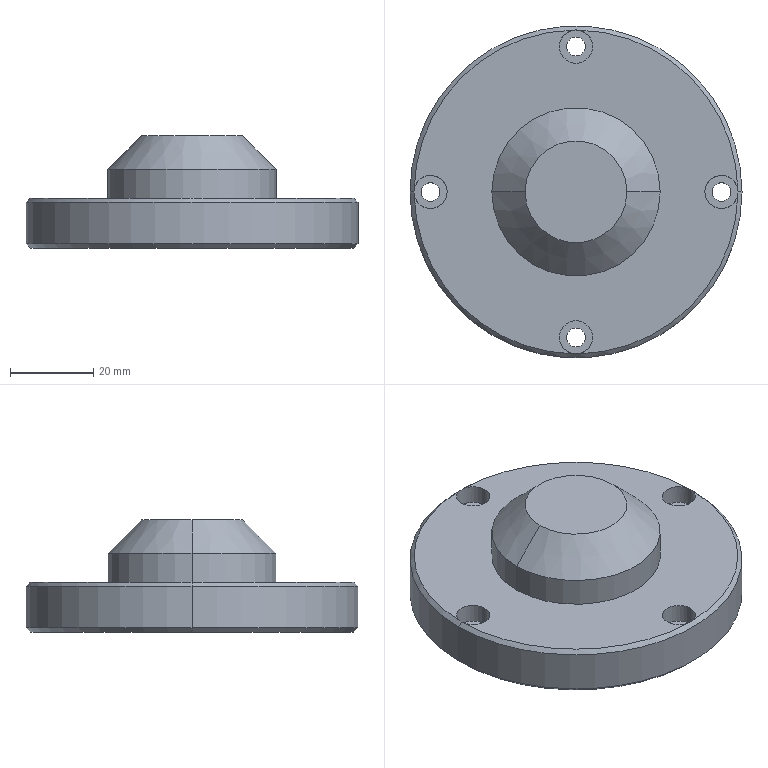Part | STEP file | TJ-DHQM-004-009 | 1 solid | 33 faces | box 79.9 x 79.9 x 27 mm | volume 74312 mm3 | cylinder 20 | plane 7 | cone 6 | commonest cylinder face diameters 4.5 x8 8 x8 40.5 x2 79.9 x2
STEP:
#1=CARTESIAN_POINT('',(12.25,0.,27.));
#2=VERTEX_POINT('',#1);
#3=CARTESIAN_POINT('',(-12.25,0.,27.));
#4=VERTEX_POINT('',#3);
#5=CARTESIAN_POINT('',(0.,0.,27.));
#6=DIRECTION('',(0.,0.,1.));
#7=DIRECTION('',(1.,0.,0.));
#8=AXIS2_PLACEMENT_3D('',#5,#6,#7);
#9=CIRCLE('',#8,12.25);
#10=EDGE_CURVE('',#2,#4,#9,.T.);
#11=ORIENTED_EDGE('',*,*,#10,.F.);
#12=CARTESIAN_POINT('',(20.25,0.,19.));
#13=VERTEX_POINT('',#12);
#14=CARTESIAN_POINT('',(12.25,0.,27.));
#15=DIRECTION('',(0.7071,0.,-0.7071));
#16=VECTOR('',#15,1000.);
#17=LINE('',#14,#16);
#18=EDGE_CURVE('',#2,#13,#17,.T.);
#19=ORIENTED_EDGE('',*,*,#18,.T.);
#20=CARTESIAN_POINT('',(-20.25,0.,19.));
#21=VERTEX_POINT('',#20);
#22=CARTESIAN_POINT('',(0.,0.,19.));
#23=DIRECTION('',(0.,0.,-1.));
#24=DIRECTION('',(1.,0.,0.));
#25=AXIS2_PLACEMENT_3D('',#22,#23,#24);
#26=CIRCLE('',#25,20.25);
#27=EDGE_CURVE('',#21,#13,#26,.T.);
#28=ORIENTED_EDGE('',*,*,#27,.F.);
#29=CARTESIAN_POINT('',(-12.25,0.,27.));
#30=DIRECTION('',(-0.7071,0.,-0.7071));
#31=VECTOR('',#30,1000.);
#32=LINE('',#29,#31);
#33=EDGE_CURVE('',#4,#21,#32,.T.);
#34=ORIENTED_EDGE('',*,*,#33,.F.);
#35=EDGE_LOOP('',(#11,#19,#28,#34));
#36=FACE_OUTER_BOUND('',#35,.T.);
#37=CARTESIAN_POINT('',(0.,0.,27.));
#38=DIRECTION('',(0.,0.,-1.));
#39=DIRECTION('',(-1.,0.,0.));
#40=AXIS2_PLACEMENT_3D('',#37,#38,#39);
#41=CONICAL_SURFACE('',#40,12.25,0.7854);
#42=ADVANCED_FACE('',(#36),#41,.T.);
#43=ORIENTED_EDGE('',*,*,#27,.T.);
#44=CARTESIAN_POINT('',(20.25,0.,12.));
#45=VERTEX_POINT('',#44);
#46=CARTESIAN_POINT('',(20.25,0.,27.));
#47=DIRECTION('',(0.,0.,-1.));
#48=VECTOR('',#47,1000.);
#49=LINE('',#46,#48);
#50=EDGE_CURVE('',#13,#45,#49,.T.);
#51=ORIENTED_EDGE('',*,*,#50,.T.);
#52=CARTESIAN_POINT('',(-20.25,0.,12.));
#53=VERTEX_POINT('',#52);
#54=CARTESIAN_POINT('',(0.,0.,12.));
#55=DIRECTION('',(0.,0.,1.));
#56=DIRECTION('',(1.,0.,0.));
#57=AXIS2_PLACEMENT_3D('',#54,#55,#56);
#58=CIRCLE('',#57,20.25);
#59=EDGE_CURVE('',#45,#53,#58,.T.);
#60=ORIENTED_EDGE('',*,*,#59,.T.);
#61=CARTESIAN_POINT('',(-20.25,0.,27.));
#62=DIRECTION('',(0.,0.,-1.));
#63=VECTOR('',#62,1000.);
#64=LINE('',#61,#63);
#65=EDGE_CURVE('',#21,#53,#64,.T.);
#66=ORIENTED_EDGE('',*,*,#65,.F.);
#67=EDGE_LOOP('',(#43,#51,#60,#66));
#68=FACE_OUTER_BOUND('',#67,.T.);
#69=CARTESIAN_POINT('',(0.,0.,27.));
#70=DIRECTION('',(0.,0.,-1.));
#71=DIRECTION('',(-1.,0.,0.));
#72=AXIS2_PLACEMENT_3D('',#69,#70,#71);
#73=CYLINDRICAL_SURFACE('',#72,20.25);
#74=ADVANCED_FACE('',(#68),#73,.T.);
#75=CARTESIAN_POINT('',(-4.,35.,7.4));
#76=VERTEX_POINT('',#75);
#77=CARTESIAN_POINT('',(4.,35.,7.4));
#78=VERTEX_POINT('',#77);
#79=CARTESIAN_POINT('',(0.,35.,7.4));
#80=DIRECTION('',(0.,0.,1.));
#81=DIRECTION('',(1.,0.,0.));
#82=AXIS2_PLACEMENT_3D('',#79,#80,#81);
#83=CIRCLE('',#82,4.);
#84=EDGE_CURVE('',#76,#78,#83,.T.);
#85=ORIENTED_EDGE('',*,*,#84,.F.);
#86=CARTESIAN_POINT('',(-4.,35.,12.));
#87=VERTEX_POINT('',#86);
#88=CARTESIAN_POINT('',(-4.,35.,12.));
#89=DIRECTION('',(0.,0.,1.));
#90=VECTOR('',#89,1000.);
#91=LINE('',#88,#90);
#92=EDGE_CURVE('',#76,#87,#91,.T.);
#93=ORIENTED_EDGE('',*,*,#92,.T.);
#94=CARTESIAN_POINT('',(4.,35.,12.));
#95=VERTEX_POINT('',#94);
#96=CARTESIAN_POINT('',(0.,35.,12.));
#97=DIRECTION('',(0.,0.,1.));
#98=DIRECTION('',(1.,0.,0.));
#99=AXIS2_PLACEMENT_3D('',#96,#97,#98);
#100=CIRCLE('',#99,4.);
#101=EDGE_CURVE('',#87,#95,#100,.T.);
#102=ORIENTED_EDGE('',*,*,#101,.T.);
#103=CARTESIAN_POINT('',(4.,35.,12.));
#104=DIRECTION('',(0.,0.,1.));
#105=VECTOR('',#104,1000.);
#106=LINE('',#103,#105);
#107=EDGE_CURVE('',#78,#95,#106,.T.);
#108=ORIENTED_EDGE('',*,*,#107,.F.);
#109=EDGE_LOOP('',(#85,#93,#102,#108));
#110=FACE_OUTER_BOUND('',#109,.T.);
#111=CARTESIAN_POINT('',(0.,35.,12.));
#112=DIRECTION('',(0.,0.,1.));
#113=DIRECTION('',(1.,0.,0.));
#114=AXIS2_PLACEMENT_3D('',#111,#112,#113);
#115=CYLINDRICAL_SURFACE('',#114,4.);
#116=ADVANCED_FACE('',(#110),#115,.F.);
#117=CARTESIAN_POINT('',(-2.25,35.,0.));
#118=VERTEX_POINT('',#117);
#119=CARTESIAN_POINT('',(2.25,35.,0.));
#120=VERTEX_POINT('',#119);
#121=CARTESIAN_POINT('',(0.,35.,0.));
#122=DIRECTION('',(0.,0.,1.));
#123=DIRECTION('',(1.,0.,0.));
#124=AXIS2_PLACEMENT_3D('',#121,#122,#123);
#125=CIRCLE('',#124,2.25);
#126=EDGE_CURVE('',#118,#120,#125,.T.);
#127=ORIENTED_EDGE('',*,*,#126,.F.);
#128=CARTESIAN_POINT('',(-2.25,35.,7.4));
#129=VERTEX_POINT('',#128);
#130=CARTESIAN_POINT('',(-2.25,35.,12.));
#131=DIRECTION('',(0.,0.,1.));
#132=VECTOR('',#131,1000.);
#133=LINE('',#130,#132);
#134=EDGE_CURVE('',#118,#129,#133,.T.);
#135=ORIENTED_EDGE('',*,*,#134,.T.);
#136=CARTESIAN_POINT('',(2.25,35.,7.4));
#137=VERTEX_POINT('',#136);
#138=CARTESIAN_POINT('',(0.,35.,7.4));
#139=DIRECTION('',(0.,0.,1.));
#140=DIRECTION('',(1.,0.,0.));
#141=AXIS2_PLACEMENT_3D('',#138,#139,#140);
#142=CIRCLE('',#141,2.25);
#143=EDGE_CURVE('',#129,#137,#142,.T.);
#144=ORIENTED_EDGE('',*,*,#143,.T.);
#145=CARTESIAN_POINT('',(2.25,35.,12.));
#146=DIRECTION('',(0.,0.,1.));
#147=VECTOR('',#146,1000.);
#148=LINE('',#145,#147);
#149=EDGE_CURVE('',#120,#137,#148,.T.);
#150=ORIENTED_EDGE('',*,*,#149,.F.);
#151=EDGE_LOOP('',(#127,#135,#144,#150));
#152=FACE_OUTER_BOUND('',#151,.T.);
#153=CARTESIAN_POINT('',(0.,35.,12.));
#154=DIRECTION('',(0.,0.,1.));
#155=DIRECTION('',(1.,0.,0.));
#156=AXIS2_PLACEMENT_3D('',#153,#154,#155);
#157=CYLINDRICAL_SURFACE('',#156,2.25);
#158=ADVANCED_FACE('',(#152),#157,.F.);
#159=CARTESIAN_POINT('',(-39.,0.,7.4));
#160=VERTEX_POINT('',#159);
#161=CARTESIAN_POINT('',(-31.,0.,7.4));
#162=VERTEX_POINT('',#161);
#163=CARTESIAN_POINT('',(-35.,0.,7.4));
#164=DIRECTION('',(0.,0.,1.));
#165=DIRECTION('',(1.,0.,0.));
#166=AXIS2_PLACEMENT_3D('',#163,#164,#165);
#167=CIRCLE('',#166,4.);
#168=EDGE_CURVE('',#160,#162,#167,.T.);
#169=ORIENTED_EDGE('',*,*,#168,.F.);
#170=CARTESIAN_POINT('',(-39.,0.,11.95));
#171=VERTEX_POINT('',#170);
#172=CARTESIAN_POINT('',(-39.,0.,12.));
#173=DIRECTION('',(0.,0.,1.));
#174=VECTOR('',#173,1000.);
#175=LINE('',#172,#174);
#176=EDGE_CURVE('',#160,#171,#175,.T.);
#177=ORIENTED_EDGE('',*,*,#176,.T.);
#178=CARTESIAN_POINT('',(-38.944,-0.6651,12.));
#179=VERTEX_POINT('',#178);
#180=CARTESIAN_POINT('',(-39.,0.,11.95));
#181=CARTESIAN_POINT('',(-39.,-0.2216,11.95));
#182=CARTESIAN_POINT('',(-38.981,-0.4461,11.967));
#183=CARTESIAN_POINT('',(-38.944,-0.6651,12.));
#184=B_SPLINE_CURVE_WITH_KNOTS('',3,(#180,#181,#182,#183),.UNSPECIFIED.,.F.,.F.,(4,4),(0.0006695,0.001333),.UNSPECIFIED.);
#185=EDGE_CURVE('',#171,#179,#184,.T.);
#186=ORIENTED_EDGE('',*,*,#185,.T.);
#187=CARTESIAN_POINT('',(-31.,0.,12.));
#188=VERTEX_POINT('',#187);
#189=CARTESIAN_POINT('',(-35.,0.,12.));
#190=DIRECTION('',(0.,0.,1.));
#191=DIRECTION('',(1.,0.,0.));
#192=AXIS2_PLACEMENT_3D('',#189,#190,#191);
#193=CIRCLE('',#192,4.);
#194=EDGE_CURVE('',#179,#188,#193,.T.);
#195=ORIENTED_EDGE('',*,*,#194,.T.);
#196=CARTESIAN_POINT('',(-31.,0.,12.));
#197=DIRECTION('',(0.,0.,1.));
#198=VECTOR('',#197,1000.);
#199=LINE('',#196,#198);
#200=EDGE_CURVE('',#162,#188,#199,.T.);
#201=ORIENTED_EDGE('',*,*,#200,.F.);
#202=EDGE_LOOP('',(#169,#177,#186,#195,#201));
#203=FACE_OUTER_BOUND('',#202,.T.);
#204=CARTESIAN_POINT('',(-35.,0.,12.));
#205=DIRECTION('',(0.,0.,1.));
#206=DIRECTION('',(1.,0.,0.));
#207=AXIS2_PLACEMENT_3D('',#204,#205,#206);
#208=CYLINDRICAL_SURFACE('',#207,4.);
#209=ADVANCED_FACE('',(#203),#208,.F.);
#210=CARTESIAN_POINT('',(-37.25,0.,0.));
#211=VERTEX_POINT('',#210);
#212=CARTESIAN_POINT('',(-32.75,0.,0.));
#213=VERTEX_POINT('',#212);
#214=CARTESIAN_POINT('',(-35.,0.,0.));
#215=DIRECTION('',(0.,0.,1.));
#216=DIRECTION('',(1.,0.,0.));
#217=AXIS2_PLACEMENT_3D('',#214,#215,#216);
#218=CIRCLE('',#217,2.25);
#219=EDGE_CURVE('',#211,#213,#218,.T.);
#220=ORIENTED_EDGE('',*,*,#219,.F.);
#221=CARTESIAN_POINT('',(-37.25,0.,7.4));
#222=VERTEX_POINT('',#221);
#223=CARTESIAN_POINT('',(-37.25,0.,12.));
#224=DIRECTION('',(0.,0.,1.));
#225=VECTOR('',#224,1000.);
#226=LINE('',#223,#225);
#227=EDGE_CURVE('',#211,#222,#226,.T.);
#228=ORIENTED_EDGE('',*,*,#227,.T.);
#229=CARTESIAN_POINT('',(-32.75,0.,7.4));
#230=VERTEX_POINT('',#229);
#231=CARTESIAN_POINT('',(-35.,0.,7.4));
#232=DIRECTION('',(0.,0.,1.));
#233=DIRECTION('',(1.,0.,0.));
#234=AXIS2_PLACEMENT_3D('',#231,#232,#233);
#235=CIRCLE('',#234,2.25);
#236=EDGE_CURVE('',#222,#230,#235,.T.);
#237=ORIENTED_EDGE('',*,*,#236,.T.);
#238=CARTESIAN_POINT('',(-32.75,0.,12.));
#239=DIRECTION('',(0.,0.,1.));
#240=VECTOR('',#239,1000.);
#241=LINE('',#238,#240);
#242=EDGE_CURVE('',#213,#230,#241,.T.);
#243=ORIENTED_EDGE('',*,*,#242,.F.);
#244=EDGE_LOOP('',(#220,#228,#237,#243));
#245=FACE_OUTER_BOUND('',#244,.T.);
#246=CARTESIAN_POINT('',(-35.,0.,12.));
#247=DIRECTION('',(0.,0.,1.));
#248=DIRECTION('',(1.,0.,0.));
#249=AXIS2_PLACEMENT_3D('',#246,#247,#248);
#250=CYLINDRICAL_SURFACE('',#249,2.25);
#251=ADVANCED_FACE('',(#245),#250,.F.);
#252=CARTESIAN_POINT('',(-4.,-35.,7.4));
#253=VERTEX_POINT('',#252);
#254=CARTESIAN_POINT('',(4.,-35.,7.4));
#255=VERTEX_POINT('',#254);
#256=CARTESIAN_POINT('',(0.,-35.,7.4));
#257=DIRECTION('',(0.,0.,1.));
#258=DIRECTION('',(1.,0.,0.));
#259=AXIS2_PLACEMENT_3D('',#256,#257,#258);
#260=CIRCLE('',#259,4.);
#261=EDGE_CURVE('',#253,#255,#260,.T.);
#262=ORIENTED_EDGE('',*,*,#261,.F.);
#263=CARTESIAN_POINT('',(-4.,-35.,12.));
#264=VERTEX_POINT('',#263);
#265=CARTESIAN_POINT('',(-4.,-35.,12.));
#266=DIRECTION('',(0.,0.,1.));
#267=VECTOR('',#266,1000.);
#268=LINE('',#265,#267);
#269=EDGE_CURVE('',#253,#264,#268,.T.);
#270=ORIENTED_EDGE('',*,*,#269,.T.);
#271=CARTESIAN_POINT('',(-0.6651,-38.944,12.));
#272=VERTEX_POINT('',#271);
#273=CARTESIAN_POINT('',(0.,-35.,12.));
#274=DIRECTION('',(0.,0.,1.));
#275=DIRECTION('',(1.,0.,0.));
#276=AXIS2_PLACEMENT_3D('',#273,#274,#275);
#277=CIRCLE('',#276,4.);
#278=EDGE_CURVE('',#264,#272,#277,.T.);
#279=ORIENTED_EDGE('',*,*,#278,.T.);
#280=CARTESIAN_POINT('',(0.6651,-38.944,12.));
#281=VERTEX_POINT('',#280);
#282=CARTESIAN_POINT('',(-0.6651,-38.944,12.));
#283=CARTESIAN_POINT('',(-0.4455,-38.981,11.967));
#284=CARTESIAN_POINT('',(-0.2245,-39.,11.95));
#285=CARTESIAN_POINT('',(0.2202,-39.,11.95));
#286=CARTESIAN_POINT('',(0.4454,-38.981,11.967));
#287=CARTESIAN_POINT('',(0.6651,-38.944,12.));
#288=B_SPLINE_CURVE_WITH_KNOTS('',3,(#282,#283,#284,#285,#286,#287),.UNSPECIFIED.,.F.,.F.,(4,2,4),(0.000001333,0.0006674,0.001333),.UNSPECIFIED.);
#289=EDGE_CURVE('',#272,#281,#288,.T.);
#290=ORIENTED_EDGE('',*,*,#289,.T.);
#291=CARTESIAN_POINT('',(4.,-35.,12.));
#292=VERTEX_POINT('',#291);
#293=CARTESIAN_POINT('',(0.,-35.,12.));
#294=DIRECTION('',(0.,0.,1.));
#295=DIRECTION('',(1.,0.,0.));
#296=AXIS2_PLACEMENT_3D('',#293,#294,#295);
#297=CIRCLE('',#296,4.);
#298=EDGE_CURVE('',#281,#292,#297,.T.);
#299=ORIENTED_EDGE('',*,*,#298,.T.);
#300=CARTESIAN_POINT('',(4.,-35.,12.));
#301=DIRECTION('',(0.,0.,1.));
#302=VECTOR('',#301,1000.);
#303=LINE('',#300,#302);
#304=EDGE_CURVE('',#255,#292,#303,.T.);
#305=ORIENTED_EDGE('',*,*,#304,.F.);
#306=EDGE_LOOP('',(#262,#270,#279,#290,#299,#305));
#307=FACE_OUTER_BOUND('',#306,.T.);
#308=CARTESIAN_POINT('',(0.,-35.,12.));
#309=DIRECTION('',(0.,0.,1.));
#310=DIRECTION('',(1.,0.,0.));
#311=AXIS2_PLACEMENT_3D('',#308,#309,#310);
#312=CYLINDRICAL_SURFACE('',#311,4.);
#313=ADVANCED_FACE('',(#307),#312,.F.);
#314=CARTESIAN_POINT('',(-2.25,-35.,0.));
#315=VERTEX_POINT('',#314);
#316=CARTESIAN_POINT('',(2.25,-35.,0.));
#317=VERTEX_POINT('',#316);
#318=CARTESIAN_POINT('',(0.,-35.,0.));
#319=DIRECTION('',(0.,0.,1.));
#320=DIRECTION('',(1.,0.,0.));
#321=AXIS2_PLACEMENT_3D('',#318,#319,#320);
#322=CIRCLE('',#321,2.25);
#323=EDGE_CURVE('',#315,#317,#322,.T.);
#324=ORIENTED_EDGE('',*,*,#323,.F.);
#325=CARTESIAN_POINT('',(-2.25,-35.,7.4));
#326=VERTEX_POINT('',#325);
#327=CARTESIAN_POINT('',(-2.25,-35.,12.));
#328=DIRECTION('',(0.,0.,1.));
#329=VECTOR('',#328,1000.);
#330=LINE('',#327,#329);
#331=EDGE_CURVE('',#315,#326,#330,.T.);
#332=ORIENTED_EDGE('',*,*,#331,.T.);
#333=CARTESIAN_POINT('',(2.25,-35.,7.4));
#334=VERTEX_POINT('',#333);
#335=CARTESIAN_POINT('',(0.,-35.,7.4));
#336=DIRECTION('',(0.,0.,1.));
#337=DIRECTION('',(1.,0.,0.));
#338=AXIS2_PLACEMENT_3D('',#335,#336,#337);
#339=CIRCLE('',#338,2.25);
#340=EDGE_CURVE('',#326,#334,#339,.T.);
#341=ORIENTED_EDGE('',*,*,#340,.T.);
#342=CARTESIAN_POINT('',(2.25,-35.,12.));
#343=DIRECTION('',(0.,0.,1.));
#344=VECTOR('',#343,1000.);
#345=LINE('',#342,#344);
#346=EDGE_CURVE('',#317,#334,#345,.T.);
#347=ORIENTED_EDGE('',*,*,#346,.F.);
#348=EDGE_LOOP('',(#324,#332,#341,#347));
#349=FACE_OUTER_BOUND('',#348,.T.);
#350=CARTESIAN_POINT('',(0.,-35.,12.));
#351=DIRECTION('',(0.,0.,1.));
#352=DIRECTION('',(1.,0.,0.));
#353=AXIS2_PLACEMENT_3D('',#350,#351,#352);
#354=CYLINDRICAL_SURFACE('',#353,2.25);
#355=ADVANCED_FACE('',(#349),#354,.F.);
#356=CARTESIAN_POINT('',(31.,0.,7.4));
#357=VERTEX_POINT('',#356);
#358=CARTESIAN_POINT('',(39.,0.,7.4));
#359=VERTEX_POINT('',#358);
#360=CARTESIAN_POINT('',(35.,0.,7.4));
#361=DIRECTION('',(0.,0.,1.));
#362=DIRECTION('',(1.,0.,0.));
#363=AXIS2_PLACEMENT_3D('',#360,#361,#362);
#364=CIRCLE('',#363,4.);
#365=EDGE_CURVE('',#357,#359,#364,.T.);
#366=ORIENTED_EDGE('',*,*,#365,.F.);
#367=CARTESIAN_POINT('',(31.,0.,12.));
#368=VERTEX_POINT('',#367);
#369=CARTESIAN_POINT('',(31.,0.,12.));
#370=DIRECTION('',(0.,0.,1.));
#371=VECTOR('',#370,1000.);
#372=LINE('',#369,#371);
#373=EDGE_CURVE('',#357,#368,#372,.T.);
#374=ORIENTED_EDGE('',*,*,#373,.T.);
#375=CARTESIAN_POINT('',(38.944,-0.6651,12.));
#376=VERTEX_POINT('',#375);
#377=CARTESIAN_POINT('',(35.,0.,12.));
#378=DIRECTION('',(0.,0.,1.));
#379=DIRECTION('',(1.,0.,0.));
#380=AXIS2_PLACEMENT_3D('',#377,#378,#379);
#381=CIRCLE('',#380,4.);
#382=EDGE_CURVE('',#368,#376,#381,.T.);
#383=ORIENTED_EDGE('',*,*,#382,.T.);
#384=CARTESIAN_POINT('',(39.,0.,11.95));
#385=VERTEX_POINT('',#384);
#386=CARTESIAN_POINT('',(38.944,-0.6651,12.));
#387=CARTESIAN_POINT('',(38.981,-0.4448,11.967));
#388=CARTESIAN_POINT('',(39.,-0.2231,11.95));
#389=CARTESIAN_POINT('',(39.,0.,11.95));
#390=B_SPLINE_CURVE_WITH_KNOTS('',3,(#386,#387,#388,#389),.UNSPECIFIED.,.F.,.F.,(4,4),(0.000001333,0.0006695),.UNSPECIFIED.);
#391=EDGE_CURVE('',#376,#385,#390,.T.);
#392=ORIENTED_EDGE('',*,*,#391,.T.);
#393=CARTESIAN_POINT('',(39.,0.,12.));
#394=DIRECTION('',(0.,0.,1.));
#395=VECTOR('',#394,1000.);
#396=LINE('',#393,#395);
#397=EDGE_CURVE('',#359,#385,#396,.T.);
#398=ORIENTED_EDGE('',*,*,#397,.F.);
#399=EDGE_LOOP('',(#366,#374,#383,#392,#398));
#400=FACE_OUTER_BOUND('',#399,.T.);
#401=CARTESIAN_POINT('',(35.,0.,12.));
#402=DIRECTION('',(0.,0.,1.));
#403=DIRECTION('',(1.,0.,0.));
#404=AXIS2_PLACEMENT_3D('',#401,#402,#403);
#405=CYLINDRICAL_SURFACE('',#404,4.);
#406=ADVANCED_FACE('',(#400),#405,.F.);
#407=CARTESIAN_POINT('',(32.75,0.,0.));
#408=VERTEX_POINT('',#407);
#409=CARTESIAN_POINT('',(37.25,0.,0.));
#410=VERTEX_POINT('',#409);
#411=CARTESIAN_POINT('',(35.,0.,0.));
#412=DIRECTION('',(0.,0.,1.));
#413=DIRECTION('',(1.,0.,0.));
#414=AXIS2_PLACEMENT_3D('',#411,#412,#413);
#415=CIRCLE('',#414,2.25);
#416=EDGE_CURVE('',#408,#410,#415,.T.);
#417=ORIENTED_EDGE('',*,*,#416,.F.);
#418=CARTESIAN_POINT('',(32.75,0.,7.4));
#419=VERTEX_POINT('',#418);
#420=CARTESIAN_POINT('',(32.75,0.,12.));
#421=DIRECTION('',(0.,0.,1.));
#422=VECTOR('',#421,1000.);
#423=LINE('',#420,#422);
#424=EDGE_CURVE('',#408,#419,#423,.T.);
#425=ORIENTED_EDGE('',*,*,#424,.T.);
#426=CARTESIAN_POINT('',(37.25,0.,7.4));
#427=VERTEX_POINT('',#426);
#428=CARTESIAN_POINT('',(35.,0.,7.4));
#429=DIRECTION('',(0.,0.,1.));
#430=DIRECTION('',(1.,0.,0.));
#431=AXIS2_PLACEMENT_3D('',#428,#429,#430);
#432=CIRCLE('',#431,2.25);
#433=EDGE_CURVE('',#419,#427,#432,.T.);
#434=ORIENTED_EDGE('',*,*,#433,.T.);
#435=CARTESIAN_POINT('',(37.25,0.,12.));
#436=DIRECTION('',(0.,0.,1.));
#437=VECTOR('',#436,1000.);
#438=LINE('',#435,#437);
#439=EDGE_CURVE('',#410,#427,#438,.T.);
#440=ORIENTED_EDGE('',*,*,#439,.F.);
#441=EDGE_LOOP('',(#417,#425,#434,#440));
#442=FACE_OUTER_BOUND('',#441,.T.);
#443=CARTESIAN_POINT('',(35.,0.,12.));
#444=DIRECTION('',(0.,0.,1.));
#445=DIRECTION('',(1.,0.,0.));
#446=AXIS2_PLACEMENT_3D('',#443,#444,#445);
#447=CYLINDRICAL_SURFACE('',#446,2.25);
#448=ADVANCED_FACE('',(#442),#447,.F.);
#449=CARTESIAN_POINT('',(38.944,0.6651,12.));
#450=VERTEX_POINT('',#449);
#451=CARTESIAN_POINT('',(39.,0.,11.95));
#452=CARTESIAN_POINT('',(39.,0.2216,11.95));
#453=CARTESIAN_POINT('',(38.981,0.4461,11.967));
#454=CARTESIAN_POINT('',(38.944,0.6651,12.));
#455=B_SPLINE_CURVE_WITH_KNOTS('',3,(#451,#452,#453,#454),.UNSPECIFIED.,.F.,.F.,(4,4),(0.0006695,0.001333),.UNSPECIFIED.);
#456=EDGE_CURVE('',#385,#450,#455,.T.);
#457=ORIENTED_EDGE('',*,*,#456,.F.);
#458=CARTESIAN_POINT('',(39.95,0.,11.));
#459=VERTEX_POINT('',#458);
#460=CARTESIAN_POINT('',(38.95,0.,12.));
#461=DIRECTION('',(0.7071,0.,-0.7071));
#462=VECTOR('',#461,1000.);
#463=LINE('',#460,#462);
#464=EDGE_CURVE('',#385,#459,#463,.T.);
#465=ORIENTED_EDGE('',*,*,#464,.T.);
#466=CARTESIAN_POINT('',(-39.95,0.,11.));
#467=VERTEX_POINT('',#466);
#468=CARTESIAN_POINT('',(0.,0.,11.));
#469=DIRECTION('',(0.,0.,-1.));
#470=DIRECTION('',(1.,0.,0.));
#471=AXIS2_PLACEMENT_3D('',#468,#469,#470);
#472=CIRCLE('',#471,39.95);
#473=EDGE_CURVE('',#467,#459,#472,.T.);
#474=ORIENTED_EDGE('',*,*,#473,.F.);
#475=CARTESIAN_POINT('',(-38.95,0.,12.));
#476=DIRECTION('',(-0.7071,0.,-0.7071));
#477=VECTOR('',#476,1000.);
#478=LINE('',#475,#477);
#479=EDGE_CURVE('',#171,#467,#478,.T.);
#480=ORIENTED_EDGE('',*,*,#479,.F.);
#481=CARTESIAN_POINT('',(-38.944,0.6651,12.));
#482=VERTEX_POINT('',#481);
#483=CARTESIAN_POINT('',(-38.944,0.6651,12.));
#484=CARTESIAN_POINT('',(-38.981,0.4448,11.967));
#485=CARTESIAN_POINT('',(-39.,0.2231,11.95));
#486=CARTESIAN_POINT('',(-39.,0.,11.95));
#487=B_SPLINE_CURVE_WITH_KNOTS('',3,(#483,#484,#485,#486),.UNSPECIFIED.,.F.,.F.,(4,4),(0.000001333,0.0006695),.UNSPECIFIED.);
#488=EDGE_CURVE('',#482,#171,#487,.T.);
#489=ORIENTED_EDGE('',*,*,#488,.F.);
#490=CARTESIAN_POINT('',(-0.6651,38.944,12.));
#491=VERTEX_POINT('',#490);
#492=CARTESIAN_POINT('',(0.,0.,12.));
#493=DIRECTION('',(0.,0.,1.));
#494=DIRECTION('',(1.,0.,0.));
#495=AXIS2_PLACEMENT_3D('',#492,#493,#494);
#496=CIRCLE('',#495,38.95);
#497=EDGE_CURVE('',#491,#482,#496,.T.);
#498=ORIENTED_EDGE('',*,*,#497,.F.);
#499=CARTESIAN_POINT('',(0.6651,38.944,12.));
#500=VERTEX_POINT('',#499);
#501=CARTESIAN_POINT('',(0.6651,38.944,12.));
#502=CARTESIAN_POINT('',(0.4455,38.981,11.967));
#503=CARTESIAN_POINT('',(0.2245,39.,11.95));
#504=CARTESIAN_POINT('',(-0.2202,39.,11.95));
#505=CARTESIAN_POINT('',(-0.4454,38.981,11.967));
#506=CARTESIAN_POINT('',(-0.6651,38.944,12.));
#507=B_SPLINE_CURVE_WITH_KNOTS('',3,(#501,#502,#503,#504,#505,#506),.UNSPECIFIED.,.F.,.F.,(4,2,4),(0.000001333,0.0006674,0.001333),.UNSPECIFIED.);
#508=EDGE_CURVE('',#500,#491,#507,.T.);
#509=ORIENTED_EDGE('',*,*,#508,.F.);
#510=CARTESIAN_POINT('',(0.,0.,12.));
#511=DIRECTION('',(0.,0.,1.));
#512=DIRECTION('',(1.,0.,0.));
#513=AXIS2_PLACEMENT_3D('',#510,#511,#512);
#514=CIRCLE('',#513,38.95);
#515=EDGE_CURVE('',#450,#500,#514,.T.);
#516=ORIENTED_EDGE('',*,*,#515,.F.);
#517=EDGE_LOOP('',(#457,#465,#474,#480,#489,#498,#509,#516));
#518=FACE_OUTER_BOUND('',#517,.T.);
#519=CARTESIAN_POINT('',(0.,0.,12.));
#520=DIRECTION('',(0.,0.,-1.));
#521=DIRECTION('',(-1.,0.,0.));
#522=AXIS2_PLACEMENT_3D('',#519,#520,#521);
#523=CONICAL_SURFACE('',#522,38.95,0.7854);
#524=ADVANCED_FACE('',(#518),#523,.T.);
#525=CARTESIAN_POINT('',(-38.95,0.,0.));
#526=VERTEX_POINT('',#525);
#527=CARTESIAN_POINT('',(38.95,0.,0.));
#528=VERTEX_POINT('',#527);
#529=CARTESIAN_POINT('',(0.,0.,0.));
#530=DIRECTION('',(0.,0.,-1.));
#531=DIRECTION('',(1.,0.,0.));
#532=AXIS2_PLACEMENT_3D('',#529,#530,#531);
#533=CIRCLE('',#532,38.95);
#534=EDGE_CURVE('',#526,#528,#533,.T.);
#535=ORIENTED_EDGE('',*,*,#534,.F.);
#536=CARTESIAN_POINT('',(-39.95,0.,1.));
#537=VERTEX_POINT('',#536);
#538=CARTESIAN_POINT('',(-39.95,0.,1.));
#539=DIRECTION('',(-0.7071,0.,0.7071));
#540=VECTOR('',#539,1000.);
#541=LINE('',#538,#540);
#542=EDGE_CURVE('',#526,#537,#541,.T.);
#543=ORIENTED_EDGE('',*,*,#542,.T.);
#544=CARTESIAN_POINT('',(39.95,0.,1.));
#545=VERTEX_POINT('',#544);
#546=CARTESIAN_POINT('',(0.,0.,1.));
#547=DIRECTION('',(0.,0.,1.));
#548=DIRECTION('',(1.,0.,0.));
#549=AXIS2_PLACEMENT_3D('',#546,#547,#548);
#550=CIRCLE('',#549,39.95);
#551=EDGE_CURVE('',#545,#537,#550,.T.);
#552=ORIENTED_EDGE('',*,*,#551,.F.);
#553=CARTESIAN_POINT('',(39.95,0.,1.));
#554=DIRECTION('',(0.7071,0.,0.7071));
#555=VECTOR('',#554,1000.);
#556=LINE('',#553,#555);
#557=EDGE_CURVE('',#528,#545,#556,.T.);
#558=ORIENTED_EDGE('',*,*,#557,.F.);
#559=EDGE_LOOP('',(#535,#543,#552,#558));
#560=FACE_OUTER_BOUND('',#559,.T.);
#561=CARTESIAN_POINT('',(0.,0.,1.));
#562=DIRECTION('',(0.,0.,1.));
#563=DIRECTION('',(1.,0.,0.));
#564=AXIS2_PLACEMENT_3D('',#561,#562,#563);
#565=CONICAL_SURFACE('',#564,39.95,0.7854);
#566=ADVANCED_FACE('',(#560),#565,.T.);
#567=ORIENTED_EDGE('',*,*,#473,.T.);
#568=CARTESIAN_POINT('',(39.95,0.,12.));
#569=DIRECTION('',(0.,0.,-1.));
#570=VECTOR('',#569,1000.);
#571=LINE('',#568,#570);
#572=EDGE_CURVE('',#459,#545,#571,.T.);
#573=ORIENTED_EDGE('',*,*,#572,.T.);
#574=ORIENTED_EDGE('',*,*,#551,.T.);
#575=CARTESIAN_POINT('',(-39.95,0.,12.));
#576=DIRECTION('',(0.,0.,-1.));
#577=VECTOR('',#576,1000.);
#578=LINE('',#575,#577);
#579=EDGE_CURVE('',#467,#537,#578,.T.);
#580=ORIENTED_EDGE('',*,*,#579,.F.);
#581=EDGE_LOOP('',(#567,#573,#574,#580));
#582=FACE_OUTER_BOUND('',#581,.T.);
#583=CARTESIAN_POINT('',(0.,0.,12.));
#584=DIRECTION('',(0.,0.,-1.));
#585=DIRECTION('',(-1.,0.,0.));
#586=AXIS2_PLACEMENT_3D('',#583,#584,#585);
#587=CYLINDRICAL_SURFACE('',#586,39.95);
#588=ADVANCED_FACE('',(#582),#587,.T.);
#589=ORIENTED_EDGE('',*,*,#572,.F.);
#590=CARTESIAN_POINT('',(0.,0.,11.));
#591=DIRECTION('',(0.,0.,-1.));
#592=DIRECTION('',(1.,0.,0.));
#593=AXIS2_PLACEMENT_3D('',#590,#591,#592);
#594=CIRCLE('',#593,39.95);
#595=EDGE_CURVE('',#459,#467,#594,.T.);
#596=ORIENTED_EDGE('',*,*,#595,.T.);
#597=ORIENTED_EDGE('',*,*,#579,.T.);
#598=CARTESIAN_POINT('',(0.,0.,1.));
#599=DIRECTION('',(0.,0.,1.));
#600=DIRECTION('',(1.,0.,0.));
#601=AXIS2_PLACEMENT_3D('',#598,#599,#600);
#602=CIRCLE('',#601,39.95);
#603=EDGE_CURVE('',#537,#545,#602,.T.);
#604=ORIENTED_EDGE('',*,*,#603,.T.);
#605=EDGE_LOOP('',(#589,#596,#597,#604));
#606=FACE_OUTER_BOUND('',#605,.T.);
#607=CARTESIAN_POINT('',(0.,0.,12.));
#608=DIRECTION('',(0.,0.,-1.));
#609=DIRECTION('',(-1.,0.,0.));
#610=AXIS2_PLACEMENT_3D('',#607,#608,#609);
#611=CYLINDRICAL_SURFACE('',#610,39.95);
#612=ADVANCED_FACE('',(#606),#611,.T.);
#613=CARTESIAN_POINT('',(0.,0.,12.));
#614=DIRECTION('',(0.,0.,1.));
#615=DIRECTION('',(1.,0.,0.));
#616=AXIS2_PLACEMENT_3D('',#613,#614,#615);
#617=CIRCLE('',#616,20.25);
#618=EDGE_CURVE('',#53,#45,#617,.T.);
#619=ORIENTED_EDGE('',*,*,#618,.F.);
#620=ORIENTED_EDGE('',*,*,#59,.F.);
#621=EDGE_LOOP('',(#619,#620));
#622=FACE_BOUND('',#621,.T.);
#623=CARTESIAN_POINT('',(0.,35.,12.));
#624=DIRECTION('',(0.,0.,1.));
#625=DIRECTION('',(1.,0.,0.));
#626=AXIS2_PLACEMENT_3D('',#623,#624,#625);
#627=CIRCLE('',#626,4.);
#628=EDGE_CURVE('',#491,#87,#627,.T.);
#629=ORIENTED_EDGE('',*,*,#628,.F.);
#630=ORIENTED_EDGE('',*,*,#497,.T.);
#631=CARTESIAN_POINT('',(-35.,0.,12.));
#632=DIRECTION('',(0.,0.,1.));
#633=DIRECTION('',(1.,0.,0.));
#634=AXIS2_PLACEMENT_3D('',#631,#632,#633);
#635=CIRCLE('',#634,4.);
#636=EDGE_CURVE('',#188,#482,#635,.T.);
#637=ORIENTED_EDGE('',*,*,#636,.F.);
#638=ORIENTED_EDGE('',*,*,#194,.F.);
#639=CARTESIAN_POINT('',(0.,0.,12.));
#640=DIRECTION('',(0.,0.,1.));
#641=DIRECTION('',(1.,0.,0.));
#642=AXIS2_PLACEMENT_3D('',#639,#640,#641);
#643=CIRCLE('',#642,38.95);
#644=EDGE_CURVE('',#179,#272,#643,.T.);
#645=ORIENTED_EDGE('',*,*,#644,.T.);
#646=ORIENTED_EDGE('',*,*,#278,.F.);
#647=CARTESIAN_POINT('',(0.,-35.,12.));
#648=DIRECTION('',(0.,0.,1.));
#649=DIRECTION('',(1.,0.,0.));
#650=AXIS2_PLACEMENT_3D('',#647,#648,#649);
#651=CIRCLE('',#650,4.);
#652=EDGE_CURVE('',#292,#264,#651,.T.);
#653=ORIENTED_EDGE('',*,*,#652,.F.);
#654=ORIENTED_EDGE('',*,*,#298,.F.);
#655=CARTESIAN_POINT('',(0.,0.,12.));
#656=DIRECTION('',(0.,0.,1.));
#657=DIRECTION('',(1.,0.,0.));
#658=AXIS2_PLACEMENT_3D('',#655,#656,#657);
#659=CIRCLE('',#658,38.95);
#660=EDGE_CURVE('',#281,#376,#659,.T.);
#661=ORIENTED_EDGE('',*,*,#660,.T.);
#662=ORIENTED_EDGE('',*,*,#382,.F.);
#663=CARTESIAN_POINT('',(35.,0.,12.));
#664=DIRECTION('',(0.,0.,1.));
#665=DIRECTION('',(1.,0.,0.));
#666=AXIS2_PLACEMENT_3D('',#663,#664,#665);
#667=CIRCLE('',#666,4.);
#668=EDGE_CURVE('',#450,#368,#667,.T.);
#669=ORIENTED_EDGE('',*,*,#668,.F.);
#670=ORIENTED_EDGE('',*,*,#515,.T.);
#671=CARTESIAN_POINT('',(0.,35.,12.));
#672=DIRECTION('',(0.,0.,1.));
#673=DIRECTION('',(1.,0.,0.));
#674=AXIS2_PLACEMENT_3D('',#671,#672,#673);
#675=CIRCLE('',#674,4.);
#676=EDGE_CURVE('',#95,#500,#675,.T.);
#677=ORIENTED_EDGE('',*,*,#676,.F.);
#678=ORIENTED_EDGE('',*,*,#101,.F.);
#679=EDGE_LOOP('',(#629,#630,#637,#638,#645,#646,#653,#654,#661,#662,#669,#670,#677,#678));
#680=FACE_OUTER_BOUND('',#679,.T.);
#681=CARTESIAN_POINT('',(0.,0.,12.));
#682=DIRECTION('',(0.,0.,1.));
#683=DIRECTION('',(1.,0.,0.));
#684=AXIS2_PLACEMENT_3D('',#681,#682,#683);
#685=PLANE('',#684);
#686=ADVANCED_FACE('',(#622,#680),#685,.T.);
#687=CARTESIAN_POINT('',(0.,35.,0.));
#688=DIRECTION('',(0.,0.,1.));
#689=DIRECTION('',(1.,0.,0.));
#690=AXIS2_PLACEMENT_3D('',#687,#688,#689);
#691=CIRCLE('',#690,2.25);
#692=EDGE_CURVE('',#120,#118,#691,.T.);
#693=ORIENTED_EDGE('',*,*,#692,.T.);
#694=ORIENTED_EDGE('',*,*,#126,.T.);
#695=EDGE_LOOP('',(#693,#694));
#696=FACE_BOUND('',#695,.T.);
#697=CARTESIAN_POINT('',(-35.,0.,0.));
#698=DIRECTION('',(0.,0.,1.));
#699=DIRECTION('',(1.,0.,0.));
#700=AXIS2_PLACEMENT_3D('',#697,#698,#699);
#701=CIRCLE('',#700,2.25);
#702=EDGE_CURVE('',#213,#211,#701,.T.);
#703=ORIENTED_EDGE('',*,*,#702,.T.);
#704=ORIENTED_EDGE('',*,*,#219,.T.);
#705=EDGE_LOOP('',(#703,#704));
#706=FACE_BOUND('',#705,.T.);
#707=CARTESIAN_POINT('',(0.,-35.,0.));
#708=DIRECTION('',(0.,0.,1.));
#709=DIRECTION('',(1.,0.,0.));
#710=AXIS2_PLACEMENT_3D('',#707,#708,#709);
#711=CIRCLE('',#710,2.25);
#712=EDGE_CURVE('',#317,#315,#711,.T.);
#713=ORIENTED_EDGE('',*,*,#712,.T.);
#714=ORIENTED_EDGE('',*,*,#323,.T.);
#715=EDGE_LOOP('',(#713,#714));
#716=FACE_BOUND('',#715,.T.);
#717=CARTESIAN_POINT('',(35.,0.,0.));
#718=DIRECTION('',(0.,0.,1.));
#719=DIRECTION('',(1.,0.,0.));
#720=AXIS2_PLACEMENT_3D('',#717,#718,#719);
#721=CIRCLE('',#720,2.25);
#722=EDGE_CURVE('',#410,#408,#721,.T.);
#723=ORIENTED_EDGE('',*,*,#722,.T.);
#724=ORIENTED_EDGE('',*,*,#416,.T.);
#725=EDGE_LOOP('',(#723,#724));
#726=FACE_BOUND('',#725,.T.);
#727=CARTESIAN_POINT('',(0.,0.,0.));
#728=DIRECTION('',(0.,0.,-1.));
#729=DIRECTION('',(1.,0.,0.));
#730=AXIS2_PLACEMENT_3D('',#727,#728,#729);
#731=CIRCLE('',#730,38.95);
#732=EDGE_CURVE('',#528,#526,#731,.T.);
#733=ORIENTED_EDGE('',*,*,#732,.T.);
#734=ORIENTED_EDGE('',*,*,#534,.T.);
#735=EDGE_LOOP('',(#733,#734));
#736=FACE_OUTER_BOUND('',#735,.T.);
#737=CARTESIAN_POINT('',(0.,0.,0.));
#738=DIRECTION('',(0.,0.,1.));
#739=DIRECTION('',(1.,0.,0.));
#740=AXIS2_PLACEMENT_3D('',#737,#738,#739);
#741=PLANE('',#740);
#742=ADVANCED_FACE('',(#696,#706,#716,#726,#736),#741,.F.);
#743=ORIENTED_EDGE('',*,*,#542,.F.);
#744=ORIENTED_EDGE('',*,*,#732,.F.);
#745=ORIENTED_EDGE('',*,*,#557,.T.);
#746=ORIENTED_EDGE('',*,*,#603,.F.);
#747=EDGE_LOOP('',(#743,#744,#745,#746));
#748=FACE_OUTER_BOUND('',#747,.T.);
#749=CARTESIAN_POINT('',(0.,0.,1.));
#750=DIRECTION('',(0.,0.,1.));
#751=DIRECTION('',(1.,0.,0.));
#752=AXIS2_PLACEMENT_3D('',#749,#750,#751);
#753=CONICAL_SURFACE('',#752,39.95,0.7854);
#754=ADVANCED_FACE('',(#748),#753,.T.);
#755=ORIENTED_EDGE('',*,*,#464,.F.);
#756=ORIENTED_EDGE('',*,*,#391,.F.);
#757=ORIENTED_EDGE('',*,*,#660,.F.);
#758=ORIENTED_EDGE('',*,*,#289,.F.);
#759=ORIENTED_EDGE('',*,*,#644,.F.);
#760=ORIENTED_EDGE('',*,*,#185,.F.);
#761=ORIENTED_EDGE('',*,*,#479,.T.);
#762=ORIENTED_EDGE('',*,*,#595,.F.);
#763=EDGE_LOOP('',(#755,#756,#757,#758,#759,#760,#761,#762));
#764=FACE_OUTER_BOUND('',#763,.T.);
#765=CARTESIAN_POINT('',(0.,0.,12.));
#766=DIRECTION('',(0.,0.,-1.));
#767=DIRECTION('',(-1.,0.,0.));
#768=AXIS2_PLACEMENT_3D('',#765,#766,#767);
#769=CONICAL_SURFACE('',#768,38.95,0.7854);
#770=ADVANCED_FACE('',(#764),#769,.T.);
#771=ORIENTED_EDGE('',*,*,#424,.F.);
#772=ORIENTED_EDGE('',*,*,#722,.F.);
#773=ORIENTED_EDGE('',*,*,#439,.T.);
#774=CARTESIAN_POINT('',(35.,0.,7.4));
#775=DIRECTION('',(0.,0.,1.));
#776=DIRECTION('',(1.,0.,0.));
#777=AXIS2_PLACEMENT_3D('',#774,#775,#776);
#778=CIRCLE('',#777,2.25);
#779=EDGE_CURVE('',#427,#419,#778,.T.);
#780=ORIENTED_EDGE('',*,*,#779,.T.);
#781=EDGE_LOOP('',(#771,#772,#773,#780));
#782=FACE_OUTER_BOUND('',#781,.T.);
#783=CARTESIAN_POINT('',(35.,0.,12.));
#784=DIRECTION('',(0.,0.,1.));
#785=DIRECTION('',(1.,0.,0.));
#786=AXIS2_PLACEMENT_3D('',#783,#784,#785);
#787=CYLINDRICAL_SURFACE('',#786,2.25);
#788=ADVANCED_FACE('',(#782),#787,.F.);
#789=ORIENTED_EDGE('',*,*,#779,.F.);
#790=ORIENTED_EDGE('',*,*,#433,.F.);
#791=EDGE_LOOP('',(#789,#790));
#792=FACE_BOUND('',#791,.T.);
#793=CARTESIAN_POINT('',(35.,0.,7.4));
#794=DIRECTION('',(0.,0.,1.));
#795=DIRECTION('',(1.,0.,0.));
#796=AXIS2_PLACEMENT_3D('',#793,#794,#795);
#797=CIRCLE('',#796,4.);
#798=EDGE_CURVE('',#359,#357,#797,.T.);
#799=ORIENTED_EDGE('',*,*,#798,.T.);
#800=ORIENTED_EDGE('',*,*,#365,.T.);
#801=EDGE_LOOP('',(#799,#800));
#802=FACE_OUTER_BOUND('',#801,.T.);
#803=CARTESIAN_POINT('',(37.25,0.,7.4));
#804=DIRECTION('',(0.,0.,-1.));
#805=DIRECTION('',(-1.,0.,0.));
#806=AXIS2_PLACEMENT_3D('',#803,#804,#805);
#807=PLANE('',#806);
#808=ADVANCED_FACE('',(#792,#802),#807,.F.);
#809=ORIENTED_EDGE('',*,*,#373,.F.);
#810=ORIENTED_EDGE('',*,*,#798,.F.);
#811=ORIENTED_EDGE('',*,*,#397,.T.);
#812=ORIENTED_EDGE('',*,*,#456,.T.);
#813=ORIENTED_EDGE('',*,*,#668,.T.);
#814=EDGE_LOOP('',(#809,#810,#811,#812,#813));
#815=FACE_OUTER_BOUND('',#814,.T.);
#816=CARTESIAN_POINT('',(35.,0.,12.));
#817=DIRECTION('',(0.,0.,1.));
#818=DIRECTION('',(1.,0.,0.));
#819=AXIS2_PLACEMENT_3D('',#816,#817,#818);
#820=CYLINDRICAL_SURFACE('',#819,4.);
#821=ADVANCED_FACE('',(#815),#820,.F.);
#822=ORIENTED_EDGE('',*,*,#331,.F.);
#823=ORIENTED_EDGE('',*,*,#712,.F.);
#824=ORIENTED_EDGE('',*,*,#346,.T.);
#825=CARTESIAN_POINT('',(0.,-35.,7.4));
#826=DIRECTION('',(0.,0.,1.));
#827=DIRECTION('',(1.,0.,0.));
#828=AXIS2_PLACEMENT_3D('',#825,#826,#827);
#829=CIRCLE('',#828,2.25);
#830=EDGE_CURVE('',#334,#326,#829,.T.);
#831=ORIENTED_EDGE('',*,*,#830,.T.);
#832=EDGE_LOOP('',(#822,#823,#824,#831));
#833=FACE_OUTER_BOUND('',#832,.T.);
#834=CARTESIAN_POINT('',(0.,-35.,12.));
#835=DIRECTION('',(0.,0.,1.));
#836=DIRECTION('',(1.,0.,0.));
#837=AXIS2_PLACEMENT_3D('',#834,#835,#836);
#838=CYLINDRICAL_SURFACE('',#837,2.25);
#839=ADVANCED_FACE('',(#833),#838,.F.);
#840=ORIENTED_EDGE('',*,*,#830,.F.);
#841=ORIENTED_EDGE('',*,*,#340,.F.);
#842=EDGE_LOOP('',(#840,#841));
#843=FACE_BOUND('',#842,.T.);
#844=CARTESIAN_POINT('',(0.,-35.,7.4));
#845=DIRECTION('',(0.,0.,1.));
#846=DIRECTION('',(1.,0.,0.));
#847=AXIS2_PLACEMENT_3D('',#844,#845,#846);
#848=CIRCLE('',#847,4.);
#849=EDGE_CURVE('',#255,#253,#848,.T.);
#850=ORIENTED_EDGE('',*,*,#849,.T.);
#851=ORIENTED_EDGE('',*,*,#261,.T.);
#852=EDGE_LOOP('',(#850,#851));
#853=FACE_OUTER_BOUND('',#852,.T.);
#854=CARTESIAN_POINT('',(2.25,-35.,7.4));
#855=DIRECTION('',(0.,0.,-1.));
#856=DIRECTION('',(-1.,0.,0.));
#857=AXIS2_PLACEMENT_3D('',#854,#855,#856);
#858=PLANE('',#857);
#859=ADVANCED_FACE('',(#843,#853),#858,.F.);
#860=ORIENTED_EDGE('',*,*,#269,.F.);
#861=ORIENTED_EDGE('',*,*,#849,.F.);
#862=ORIENTED_EDGE('',*,*,#304,.T.);
#863=ORIENTED_EDGE('',*,*,#652,.T.);
#864=EDGE_LOOP('',(#860,#861,#862,#863));
#865=FACE_OUTER_BOUND('',#864,.T.);
#866=CARTESIAN_POINT('',(0.,-35.,12.));
#867=DIRECTION('',(0.,0.,1.));
#868=DIRECTION('',(1.,0.,0.));
#869=AXIS2_PLACEMENT_3D('',#866,#867,#868);
#870=CYLINDRICAL_SURFACE('',#869,4.);
#871=ADVANCED_FACE('',(#865),#870,.F.);
#872=ORIENTED_EDGE('',*,*,#227,.F.);
#873=ORIENTED_EDGE('',*,*,#702,.F.);
#874=ORIENTED_EDGE('',*,*,#242,.T.);
#875=CARTESIAN_POINT('',(-35.,0.,7.4));
#876=DIRECTION('',(0.,0.,1.));
#877=DIRECTION('',(1.,0.,0.));
#878=AXIS2_PLACEMENT_3D('',#875,#876,#877);
#879=CIRCLE('',#878,2.25);
#880=EDGE_CURVE('',#230,#222,#879,.T.);
#881=ORIENTED_EDGE('',*,*,#880,.T.);
#882=EDGE_LOOP('',(#872,#873,#874,#881));
#883=FACE_OUTER_BOUND('',#882,.T.);
#884=CARTESIAN_POINT('',(-35.,0.,12.));
#885=DIRECTION('',(0.,0.,1.));
#886=DIRECTION('',(1.,0.,0.));
#887=AXIS2_PLACEMENT_3D('',#884,#885,#886);
#888=CYLINDRICAL_SURFACE('',#887,2.25);
#889=ADVANCED_FACE('',(#883),#888,.F.);
#890=ORIENTED_EDGE('',*,*,#880,.F.);
#891=ORIENTED_EDGE('',*,*,#236,.F.);
#892=EDGE_LOOP('',(#890,#891));
#893=FACE_BOUND('',#892,.T.);
#894=CARTESIAN_POINT('',(-35.,0.,7.4));
#895=DIRECTION('',(0.,0.,1.));
#896=DIRECTION('',(1.,0.,0.));
#897=AXIS2_PLACEMENT_3D('',#894,#895,#896);
#898=CIRCLE('',#897,4.);
#899=EDGE_CURVE('',#162,#160,#898,.T.);
#900=ORIENTED_EDGE('',*,*,#899,.T.);
#901=ORIENTED_EDGE('',*,*,#168,.T.);
#902=EDGE_LOOP('',(#900,#901));
#903=FACE_OUTER_BOUND('',#902,.T.);
#904=CARTESIAN_POINT('',(-32.75,0.,7.4));
#905=DIRECTION('',(0.,0.,-1.));
#906=DIRECTION('',(-1.,0.,0.));
#907=AXIS2_PLACEMENT_3D('',#904,#905,#906);
#908=PLANE('',#907);
#909=ADVANCED_FACE('',(#893,#903),#908,.F.);
#910=ORIENTED_EDGE('',*,*,#176,.F.);
#911=ORIENTED_EDGE('',*,*,#899,.F.);
#912=ORIENTED_EDGE('',*,*,#200,.T.);
#913=ORIENTED_EDGE('',*,*,#636,.T.);
#914=ORIENTED_EDGE('',*,*,#488,.T.);
#915=EDGE_LOOP('',(#910,#911,#912,#913,#914));
#916=FACE_OUTER_BOUND('',#915,.T.);
#917=CARTESIAN_POINT('',(-35.,0.,12.));
#918=DIRECTION('',(0.,0.,1.));
#919=DIRECTION('',(1.,0.,0.));
#920=AXIS2_PLACEMENT_3D('',#917,#918,#919);
#921=CYLINDRICAL_SURFACE('',#920,4.);
#922=ADVANCED_FACE('',(#916),#921,.F.);
#923=ORIENTED_EDGE('',*,*,#134,.F.);
#924=ORIENTED_EDGE('',*,*,#692,.F.);
#925=ORIENTED_EDGE('',*,*,#149,.T.);
#926=CARTESIAN_POINT('',(0.,35.,7.4));
#927=DIRECTION('',(0.,0.,1.));
#928=DIRECTION('',(1.,0.,0.));
#929=AXIS2_PLACEMENT_3D('',#926,#927,#928);
#930=CIRCLE('',#929,2.25);
#931=EDGE_CURVE('',#137,#129,#930,.T.);
#932=ORIENTED_EDGE('',*,*,#931,.T.);
#933=EDGE_LOOP('',(#923,#924,#925,#932));
#934=FACE_OUTER_BOUND('',#933,.T.);
#935=CARTESIAN_POINT('',(0.,35.,12.));
#936=DIRECTION('',(0.,0.,1.));
#937=DIRECTION('',(1.,0.,0.));
#938=AXIS2_PLACEMENT_3D('',#935,#936,#937);
#939=CYLINDRICAL_SURFACE('',#938,2.25);
#940=ADVANCED_FACE('',(#934),#939,.F.);
#941=ORIENTED_EDGE('',*,*,#931,.F.);
#942=ORIENTED_EDGE('',*,*,#143,.F.);
#943=EDGE_LOOP('',(#941,#942));
#944=FACE_BOUND('',#943,.T.);
#945=CARTESIAN_POINT('',(0.,35.,7.4));
#946=DIRECTION('',(0.,0.,1.));
#947=DIRECTION('',(1.,0.,0.));
#948=AXIS2_PLACEMENT_3D('',#945,#946,#947);
#949=CIRCLE('',#948,4.);
#950=EDGE_CURVE('',#78,#76,#949,.T.);
#951=ORIENTED_EDGE('',*,*,#950,.T.);
#952=ORIENTED_EDGE('',*,*,#84,.T.);
#953=EDGE_LOOP('',(#951,#952));
#954=FACE_OUTER_BOUND('',#953,.T.);
#955=CARTESIAN_POINT('',(2.25,35.,7.4));
#956=DIRECTION('',(0.,0.,-1.));
#957=DIRECTION('',(-1.,0.,0.));
#958=AXIS2_PLACEMENT_3D('',#955,#956,#957);
#959=PLANE('',#958);
#960=ADVANCED_FACE('',(#944,#954),#959,.F.);
#961=ORIENTED_EDGE('',*,*,#92,.F.);
#962=ORIENTED_EDGE('',*,*,#950,.F.);
#963=ORIENTED_EDGE('',*,*,#107,.T.);
#964=ORIENTED_EDGE('',*,*,#676,.T.);
#965=ORIENTED_EDGE('',*,*,#508,.T.);
#966=ORIENTED_EDGE('',*,*,#628,.T.);
#967=EDGE_LOOP('',(#961,#962,#963,#964,#965,#966));
#968=FACE_OUTER_BOUND('',#967,.T.);
#969=CARTESIAN_POINT('',(0.,35.,12.));
#970=DIRECTION('',(0.,0.,1.));
#971=DIRECTION('',(1.,0.,0.));
#972=AXIS2_PLACEMENT_3D('',#969,#970,#971);
#973=CYLINDRICAL_SURFACE('',#972,4.);
#974=ADVANCED_FACE('',(#968),#973,.F.);
#975=ORIENTED_EDGE('',*,*,#50,.F.);
#976=CARTESIAN_POINT('',(0.,0.,19.));
#977=DIRECTION('',(0.,0.,-1.));
#978=DIRECTION('',(1.,0.,0.));
#979=AXIS2_PLACEMENT_3D('',#976,#977,#978);
#980=CIRCLE('',#979,20.25);
#981=EDGE_CURVE('',#13,#21,#980,.T.);
#982=ORIENTED_EDGE('',*,*,#981,.T.);
#983=ORIENTED_EDGE('',*,*,#65,.T.);
#984=ORIENTED_EDGE('',*,*,#618,.T.);
#985=EDGE_LOOP('',(#975,#982,#983,#984));
#986=FACE_OUTER_BOUND('',#985,.T.);
#987=CARTESIAN_POINT('',(0.,0.,27.));
#988=DIRECTION('',(0.,0.,-1.));
#989=DIRECTION('',(-1.,0.,0.));
#990=AXIS2_PLACEMENT_3D('',#987,#988,#989);
#991=CYLINDRICAL_SURFACE('',#990,20.25);
#992=ADVANCED_FACE('',(#986),#991,.T.);
#993=CARTESIAN_POINT('',(0.,0.,27.));
#994=DIRECTION('',(0.,0.,1.));
#995=DIRECTION('',(1.,0.,0.));
#996=AXIS2_PLACEMENT_3D('',#993,#994,#995);
#997=CIRCLE('',#996,12.25);
#998=EDGE_CURVE('',#4,#2,#997,.T.);
#999=ORIENTED_EDGE('',*,*,#998,.T.);
#1000=ORIENTED_EDGE('',*,*,#10,.T.);
#1001=EDGE_LOOP('',(#999,#1000));
#1002=FACE_OUTER_BOUND('',#1001,.T.);
#1003=CARTESIAN_POINT('',(0.,0.,27.));
#1004=DIRECTION('',(0.,0.,1.));
#1005=DIRECTION('',(1.,0.,0.));
#1006=AXIS2_PLACEMENT_3D('',#1003,#1004,#1005);
#1007=PLANE('',#1006);
#1008=ADVANCED_FACE('',(#1002),#1007,.T.);
#1009=ORIENTED_EDGE('',*,*,#18,.F.);
#1010=ORIENTED_EDGE('',*,*,#998,.F.);
#1011=ORIENTED_EDGE('',*,*,#33,.T.);
#1012=ORIENTED_EDGE('',*,*,#981,.F.);
#1013=EDGE_LOOP('',(#1009,#1010,#1011,#1012));
#1014=FACE_OUTER_BOUND('',#1013,.T.);
#1015=CARTESIAN_POINT('',(0.,0.,27.));
#1016=DIRECTION('',(0.,0.,-1.));
#1017=DIRECTION('',(-1.,0.,0.));
#1018=AXIS2_PLACEMENT_3D('',#1015,#1016,#1017);
#1019=CONICAL_SURFACE('',#1018,12.25,0.7854);
#1020=ADVANCED_FACE('',(#1014),#1019,.T.);
#1021=CLOSED_SHELL('',(#42,#74,#116,#158,#209,#251,#313,#355,#406,#448,#524,#566,#588,#612,#686,#742,#754,#770,#788,#808,#821,#839,#859,#871,#889,#909,#922,#940,#960,#974,#992,#1008,#1020));
#1022=MANIFOLD_SOLID_BREP('',#1021);
#1023=CARTESIAN_POINT('',(0.,0.,0.));
#1024=DIRECTION('',(0.,0.,1.));
#1025=DIRECTION('',(1.,0.,0.));
#1026=AXIS2_PLACEMENT_3D('',#1023,#1024,#1025);
#1027=(LENGTH_UNIT()NAMED_UNIT(*)SI_UNIT(.MILLI.,.METRE.));
#1028=UNCERTAINTY_MEASURE_WITH_UNIT(LENGTH_MEASURE(0.00001),#1027,'','');
#1029=(NAMED_UNIT(*)PLANE_ANGLE_UNIT()SI_UNIT($,.RADIAN.));
#1030=(NAMED_UNIT(*)SI_UNIT($,.STERADIAN.)SOLID_ANGLE_UNIT());
#1031=(GEOMETRIC_REPRESENTATION_CONTEXT(3)GLOBAL_UNCERTAINTY_ASSIGNED_CONTEXT((#1028))GLOBAL_UNIT_ASSIGNED_CONTEXT((#1027,#1029,#1030))REPRESENTATION_CONTEXT('',''));
#1032=ADVANCED_BREP_SHAPE_REPRESENTATION('',(#1022,#1026),#1031);